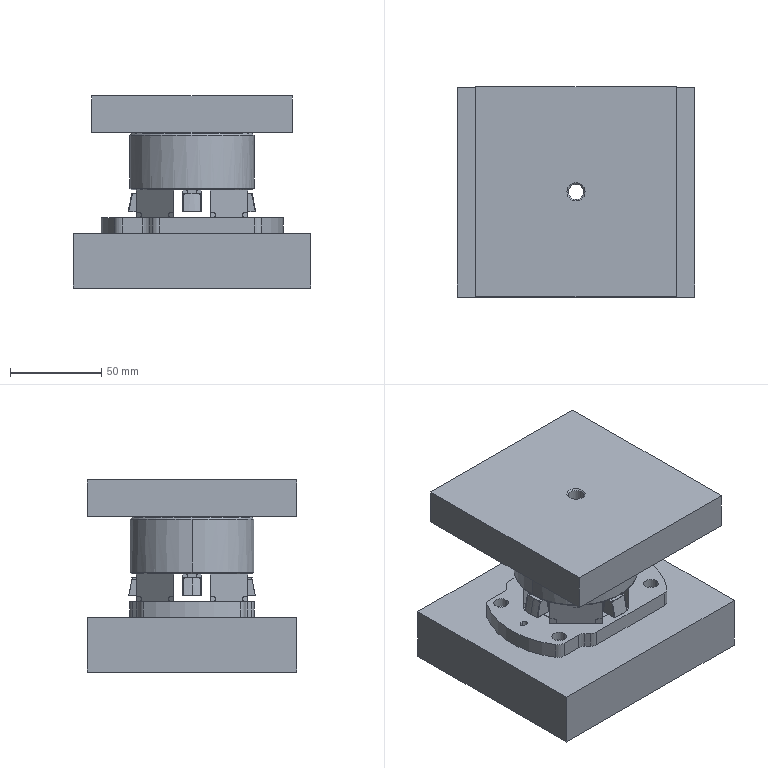NC program | NX | posted with a generic post | part box 130 x 115 x 105.2 mm
Lines 1 to 1408 of 4507:
N10 G17 G21 G94 G90
(135 , TOOL : ER25-D10-50)
N12 T04 M6
N14 G54
N16 G17 G0 G90 X-5.205 Y53.804 S5000 M3
N18 G43 Z87.387 H4
N20 G94 G1 Y7.667 Z41.249 F4500.
N22 G41 X-5.2 Y14.243 Z34.673 F2500.
N24 Y33.118 Z15.798
N26 Y34.06 Z14.855 F2292.
N28 Y35.003 Z13.913 F2083.
N30 Y35.946 Z12.97 F1875.
N32 Y36.889 Z12.027 F1667.
N34 Y37.832 Z11.084 F1458.
N36 Y38.774 Z10.141 F1250.
N38 X-10. F2500.
N40 Y37.832 Z11.084 F1250.
N42 Y36.889 Z12.027 F1667.
N44 Y35.946 Z12.97 F2083.
N46 Y14.243 Z34.673 F2500.
N48 Y7.879 Z41.037
N50 G40
N52 X-9.995 Y7.667 Z41.249
N54 X-5.205 Y6.959 Z40.542 F6000.
N56 G41 X-5.2 Y13.536 Z33.966 F2500.
N58 Y32.41 Z15.091
N60 Y33.353 Z14.148 F2292.
N62 Y34.296 Z13.206 F2083.
N64 Y35.239 Z12.263 F1875.
N66 Y36.182 Z11.32 F1667.
N68 Y37.125 Z10.377 F1458.
N70 Y38.067 Z9.434 F1250.
N72 X-10. F2500.
N74 Y37.125 Z10.377 F1250.
N76 Y36.182 Z11.32 F1667.
N78 Y35.239 Z12.263 F2083.
N80 Y13.536 Z33.966 F2500.
N82 Y7.172 Z40.33
N84 G40
N86 X-9.995 Y6.959 Z40.542
N88 X-5.205 Y6.252 Z39.835 F6000.
N90 G41 X-5.2 Y12.828 Z33.259 F2500.
N92 Y31.703 Z14.384
N94 Y32.646 Z13.441 F2292.
N96 Y33.589 Z12.498 F2083.
N98 Y34.532 Z11.556 F1875.
N100 Y35.475 Z10.613 F1667.
N102 Y36.417 Z9.67 F1458.
N104 Y37.36 Z8.727 F1250.
N106 X-10. F2500.
N108 Y36.417 Z9.67 F1250.
N110 Y35.475 Z10.613 F1667.
N112 Y34.532 Z11.556 F2083.
N114 Y12.828 Z33.259 F2500.
N116 Y6.464 Z39.623
N118 G40
N120 X-9.995 Y6.252 Z39.835
N122 X-5.205 Y5.545 Z39.128 F6000.
N124 G41 X-5.2 Y12.121 Z32.552 F2500.
N126 Y30.996 Z13.677
N128 Y31.939 Z12.734 F2292.
N130 Y32.882 Z11.791 F2083.
N132 Y33.825 Z10.849 F1875.
N134 Y34.767 Z9.906 F1667.
N136 Y35.71 Z8.963 F1458.
N138 Y36.653 Z8.02 F1250.
N140 X-10. F2500.
N142 Y35.71 Z8.963 F1250.
N144 Y34.767 Z9.906 F1667.
N146 Y33.825 Z10.849 F2083.
N148 Y12.121 Z32.552 F2500.
N150 Y5.757 Z38.916
N152 G40
N154 X-9.995 Y5.545 Z39.128
N156 X-5.205 Y4.838 Z38.421 F6000.
N158 G41 X-5.2 Y11.414 Z31.845 F2500.
N160 Y30.289 Z12.97
N162 Y31.232 Z12.027 F2292.
N164 Y32.175 Z11.084 F2083.
N166 Y33.118 Z10.141 F1875.
N168 Y34.06 Z9.199 F1667.
N170 Y35.003 Z8.256 F1458.
N172 Y35.946 Z7.313 F1250.
N174 X-10. F2500.
N176 Y35.003 Z8.256 F1250.
N178 Y34.06 Z9.199 F1667.
N180 Y33.118 Z10.141 F2083.
N182 Y11.414 Z31.845 F2500.
N184 Y5.05 Z38.209
N186 G40
N188 X-9.995 Y4.838 Z38.421
N190 X-5.205 Y4.131 Z37.714 F6000.
N192 G41 X-5.2 Y10.707 Z31.138 F2500.
N194 Y29.582 Z12.263
N196 Y30.525 Z11.32 F2292.
N198 Y31.468 Z10.377 F2083.
N200 Y32.41 Z9.434 F1875.
N202 Y33.353 Z8.492 F1667.
N204 Y34.296 Z7.549 F1458.
N206 Y35.239 Z6.606 F1250.
N208 X-10. F2500.
N210 Y34.296 Z7.549 F1250.
N212 Y33.353 Z8.492 F1667.
N214 Y32.41 Z9.434 F2083.
N216 Y10.707 Z31.138 F2500.
N218 Y4.343 Z37.502
N220 G40
N222 X-9.995 Y4.131 Z37.714
N224 X-5.205 Y3.495 Z37.077 F6000.
N226 G41 X-5.2 Y10.071 Z30.501 F2500.
N228 Y28.946 Z11.626
N230 Y29.888 Z10.684 F2292.
N232 Y30.831 Z9.741 F2083.
N234 Y31.774 Z8.798 F1875.
N236 Y32.717 Z7.855 F1667.
N238 Y33.66 Z6.912 F1458.
N240 Y34.602 Z5.969 F1250.
N242 X-10. F2500.
N244 Y33.66 Z6.912 F1250.
N246 Y32.717 Z7.855 F1667.
N248 Y31.774 Z8.798 F2083.
N250 Y10.071 Z30.501 F2500.
N252 Y3.707 Z36.865
N254 G40
N256 X-9.995 Y3.495 Z37.077
N258 G0 Y53.804 Z87.387
(PLANAR_MILL_1_5_COPY , TOOL : ER25-D10-50)
N260 X-5.205 Y-87.387
N262 Z53.804
N264 G1 Y-41.249 Z7.667 F4500.
N266 G41 X-5.2 Y-34.673 Z14.243 F2500.
N268 Y-15.798 Z33.118
N270 Y-14.855 Z34.06 F2292.
N272 Y-13.913 Z35.003 F2083.
N274 Y-12.97 Z35.946 F1875.
N276 Y-12.027 Z36.889 F1667.
N278 Y-11.084 Z37.832 F1458.
N280 Y-10.141 Z38.774 F1250.
N282 X-10. F2500.
N284 Y-11.084 Z37.832 F1250.
N286 Y-12.027 Z36.889 F1667.
N288 Y-12.97 Z35.946 F2083.
N290 Y-34.673 Z14.243 F2500.
N292 Y-41.037 Z7.879
N294 G40
N296 X-9.995 Y-41.249 Z7.667
N298 X-5.205 Y-40.542 Z6.959 F6000.
N300 G41 X-5.2 Y-33.966 Z13.536 F2500.
N302 Y-15.091 Z32.41
N304 Y-14.148 Z33.353 F2292.
N306 Y-13.206 Z34.296 F2083.
N308 Y-12.263 Z35.239 F1875.
N310 Y-11.32 Z36.182 F1667.
N312 Y-10.377 Z37.125 F1458.
N314 Y-9.434 Z38.067 F1250.
N316 X-10. F2500.
N318 Y-10.377 Z37.125 F1250.
N320 Y-11.32 Z36.182 F1667.
N322 Y-12.263 Z35.239 F2083.
N324 Y-33.966 Z13.536 F2500.
N326 Y-40.33 Z7.172
N328 G40
N330 X-9.995 Y-40.542 Z6.959
N332 X-5.205 Y-39.835 Z6.252 F6000.
N334 G41 X-5.2 Y-33.259 Z12.828 F2500.
N336 Y-14.384 Z31.703
N338 Y-13.441 Z32.646 F2292.
N340 Y-12.498 Z33.589 F2083.
N342 Y-11.556 Z34.532 F1875.
N344 Y-10.613 Z35.475 F1667.
N346 Y-9.67 Z36.417 F1458.
N348 Y-8.727 Z37.36 F1250.
N350 X-10. F2500.
N352 Y-9.67 Z36.417 F1250.
N354 Y-10.613 Z35.475 F1667.
N356 Y-11.556 Z34.532 F2083.
N358 Y-33.259 Z12.828 F2500.
N360 Y-39.623 Z6.464
N362 G40
N364 X-9.995 Y-39.835 Z6.252
N366 X-5.205 Y-39.128 Z5.545 F6000.
N368 G41 X-5.2 Y-32.552 Z12.121 F2500.
N370 Y-13.677 Z30.996
N372 Y-12.734 Z31.939 F2292.
N374 Y-11.791 Z32.882 F2083.
N376 Y-10.849 Z33.825 F1875.
N378 Y-9.906 Z34.767 F1667.
N380 Y-8.963 Z35.71 F1458.
N382 Y-8.02 Z36.653 F1250.
N384 X-10. F2500.
N386 Y-8.963 Z35.71 F1250.
N388 Y-9.906 Z34.767 F1667.
N390 Y-10.849 Z33.825 F2083.
N392 Y-32.552 Z12.121 F2500.
N394 Y-38.916 Z5.757
N396 G40
N398 X-9.995 Y-39.128 Z5.545
N400 X-5.205 Y-38.421 Z4.838 F6000.
N402 G41 X-5.2 Y-31.845 Z11.414 F2500.
N404 Y-12.97 Z30.289
N406 Y-12.027 Z31.232 F2292.
N408 Y-11.084 Z32.175 F2083.
N410 Y-10.141 Z33.118 F1875.
N412 Y-9.199 Z34.06 F1667.
N414 Y-8.256 Z35.003 F1458.
N416 Y-7.313 Z35.946 F1250.
N418 X-10. F2500.
N420 Y-8.256 Z35.003 F1250.
N422 Y-9.199 Z34.06 F1667.
N424 Y-10.141 Z33.118 F2083.
N426 Y-31.845 Z11.414 F2500.
N428 Y-38.209 Z5.05
N430 G40
N432 X-9.995 Y-38.421 Z4.838
N434 X-5.205 Y-37.714 Z4.131 F6000.
N436 G41 X-5.2 Y-31.138 Z10.707 F2500.
N438 Y-12.263 Z29.582
N440 Y-11.32 Z30.525 F2292.
N442 Y-10.377 Z31.468 F2083.
N444 Y-9.434 Z32.41 F1875.
N446 Y-8.492 Z33.353 F1667.
N448 Y-7.549 Z34.296 F1458.
N450 Y-6.606 Z35.239 F1250.
N452 X-10. F2500.
N454 Y-7.549 Z34.296 F1250.
N456 Y-8.492 Z33.353 F1667.
N458 Y-9.434 Z32.41 F2083.
N460 Y-31.138 Z10.707 F2500.
N462 Y-37.502 Z4.343
N464 G40
N466 X-9.995 Y-37.714 Z4.131
N468 X-5.205 Y-37.077 Z3.495 F6000.
N470 G41 X-5.2 Y-30.501 Z10.071 F2500.
N472 Y-11.626 Z28.946
N474 Y-10.684 Z29.888 F2292.
N476 Y-9.741 Z30.831 F2083.
N478 Y-8.798 Z31.774 F1875.
N480 Y-7.855 Z32.717 F1667.
N482 Y-6.912 Z33.66 F1458.
N484 Y-5.969 Z34.602 F1250.
N486 X-10. F2500.
N488 Y-6.912 Z33.66 F1250.
N490 Y-7.855 Z32.717 F1667.
N492 Y-8.798 Z31.774 F2083.
N494 Y-30.501 Z10.071 F2500.
N496 Y-36.865 Z3.707
N498 G40
N500 X-9.995 Y-37.077 Z3.495
N502 G0 Y-87.387 Z53.804
(PLANAR_MILL_1_5_COPY_1 , TOOL : ER25-D10-50)
N504 X-5.205 Y-53.804
N506 Z-87.387
N508 G1 Y-7.667 Z-41.249 F4500.
N510 G41 X-5.2 Y-14.243 Z-34.673 F2500.
N512 Y-33.118 Z-15.798
N514 Y-34.06 Z-14.855 F2292.
N516 Y-35.003 Z-13.913 F2083.
N518 Y-35.946 Z-12.97 F1875.
N520 Y-36.889 Z-12.027 F1667.
N522 Y-37.832 Z-11.084 F1458.
N524 Y-38.774 Z-10.141 F1250.
N526 X-10. F2500.
N528 Y-37.832 Z-11.084 F1250.
N530 Y-36.889 Z-12.027 F1667.
N532 Y-35.946 Z-12.97 F2083.
N534 Y-14.243 Z-34.673 F2500.
N536 Y-7.879 Z-41.037
N538 G40
N540 X-9.995 Y-7.667 Z-41.249
N542 X-5.205 Y-6.959 Z-40.542 F6000.
N544 G41 X-5.2 Y-13.536 Z-33.966 F2500.
N546 Y-32.41 Z-15.091
N548 Y-33.353 Z-14.148 F2292.
N550 Y-34.296 Z-13.206 F2083.
N552 Y-35.239 Z-12.263 F1875.
N554 Y-36.182 Z-11.32 F1667.
N556 Y-37.125 Z-10.377 F1458.
N558 Y-38.067 Z-9.434 F1250.
N560 X-10. F2500.
N562 Y-37.125 Z-10.377 F1250.
N564 Y-36.182 Z-11.32 F1667.
N566 Y-35.239 Z-12.263 F2083.
N568 Y-13.536 Z-33.966 F2500.
N570 Y-7.172 Z-40.33
N572 G40
N574 X-9.995 Y-6.959 Z-40.542
N576 X-5.205 Y-6.252 Z-39.835 F6000.
N578 G41 X-5.2 Y-12.828 Z-33.259 F2500.
N580 Y-31.703 Z-14.384
N582 Y-32.646 Z-13.441 F2292.
N584 Y-33.589 Z-12.498 F2083.
N586 Y-34.532 Z-11.556 F1875.
N588 Y-35.475 Z-10.613 F1667.
N590 Y-36.417 Z-9.67 F1458.
N592 Y-37.36 Z-8.727 F1250.
N594 X-10. F2500.
N596 Y-36.417 Z-9.67 F1250.
N598 Y-35.475 Z-10.613 F1667.
N600 Y-34.532 Z-11.556 F2083.
N602 Y-12.828 Z-33.259 F2500.
N604 Y-6.464 Z-39.623
N606 G40
N608 X-9.995 Y-6.252 Z-39.835
N610 X-5.205 Y-5.545 Z-39.128 F6000.
N612 G41 X-5.2 Y-12.121 Z-32.552 F2500.
N614 Y-30.996 Z-13.677
N616 Y-31.939 Z-12.734 F2292.
N618 Y-32.882 Z-11.791 F2083.
N620 Y-33.825 Z-10.849 F1875.
N622 Y-34.767 Z-9.906 F1667.
N624 Y-35.71 Z-8.963 F1458.
N626 Y-36.653 Z-8.02 F1250.
N628 X-10. F2500.
N630 Y-35.71 Z-8.963 F1250.
N632 Y-34.767 Z-9.906 F1667.
N634 Y-33.825 Z-10.849 F2083.
N636 Y-12.121 Z-32.552 F2500.
N638 Y-5.757 Z-38.916
N640 G40
N642 X-9.995 Y-5.545 Z-39.128
N644 X-5.205 Y-4.838 Z-38.421 F6000.
N646 G41 X-5.2 Y-11.414 Z-31.845 F2500.
N648 Y-30.289 Z-12.97
N650 Y-31.232 Z-12.027 F2292.
N652 Y-32.175 Z-11.084 F2083.
N654 Y-33.118 Z-10.141 F1875.
N656 Y-34.06 Z-9.199 F1667.
N658 Y-35.003 Z-8.256 F1458.
N660 Y-35.946 Z-7.313 F1250.
N662 X-10. F2500.
N664 Y-35.003 Z-8.256 F1250.
N666 Y-34.06 Z-9.199 F1667.
N668 Y-33.118 Z-10.141 F2083.
N670 Y-11.414 Z-31.845 F2500.
N672 Y-5.05 Z-38.209
N674 G40
N676 X-9.995 Y-4.838 Z-38.421
N678 X-5.205 Y-4.131 Z-37.714 F6000.
N680 G41 X-5.2 Y-10.707 Z-31.138 F2500.
N682 Y-29.582 Z-12.263
N684 Y-30.525 Z-11.32 F2292.
N686 Y-31.468 Z-10.377 F2083.
N688 Y-32.41 Z-9.434 F1875.
N690 Y-33.353 Z-8.492 F1667.
N692 Y-34.296 Z-7.549 F1458.
N694 Y-35.239 Z-6.606 F1250.
N696 X-10. F2500.
N698 Y-34.296 Z-7.549 F1250.
N700 Y-33.353 Z-8.492 F1667.
N702 Y-32.41 Z-9.434 F2083.
N704 Y-10.707 Z-31.138 F2500.
N706 Y-4.343 Z-37.502
N708 G40
N710 X-9.995 Y-4.131 Z-37.714
N712 X-5.205 Y-3.495 Z-37.077 F6000.
N714 G41 X-5.2 Y-10.071 Z-30.501 F2500.
N716 Y-28.946 Z-11.626
N718 Y-29.888 Z-10.684 F2292.
N720 Y-30.831 Z-9.741 F2083.
N722 Y-31.774 Z-8.798 F1875.
N724 Y-32.717 Z-7.855 F1667.
N726 Y-33.66 Z-6.912 F1458.
N728 Y-34.602 Z-5.969 F1250.
N730 X-10. F2500.
N732 Y-33.66 Z-6.912 F1250.
N734 Y-32.717 Z-7.855 F1667.
N736 Y-31.774 Z-8.798 F2083.
N738 Y-10.071 Z-30.501 F2500.
N740 Y-3.707 Z-36.865
N742 G40
N744 X-9.995 Y-3.495 Z-37.077
N746 G0 Y-53.804 Z-87.387
(PLANAR_MILL_1_5_COPY_2 , TOOL : ER25-D10-50)
N748 Z-53.804
N750 X-5.205 Y87.387
N752 G1 Y41.249 Z-7.667 F4500.
N754 G41 X-5.2 Y34.673 Z-14.243 F2500.
N756 Y15.798 Z-33.118
N758 Y14.855 Z-34.06 F2292.
N760 Y13.913 Z-35.003 F2083.
N762 Y12.97 Z-35.946 F1875.
N764 Y12.027 Z-36.889 F1667.
N766 Y11.084 Z-37.832 F1458.
N768 Y10.141 Z-38.774 F1250.
N770 X-10. F2500.
N772 Y11.084 Z-37.832 F1250.
N774 Y12.027 Z-36.889 F1667.
N776 Y12.97 Z-35.946 F2083.
N778 Y34.673 Z-14.243 F2500.
N780 Y41.037 Z-7.879
N782 G40
N784 X-9.995 Y41.249 Z-7.667
N786 X-5.205 Y40.542 Z-6.959 F6000.
N788 G41 X-5.2 Y33.966 Z-13.536 F2500.
N790 Y15.091 Z-32.41
N792 Y14.148 Z-33.353 F2292.
N794 Y13.206 Z-34.296 F2083.
N796 Y12.263 Z-35.239 F1875.
N798 Y11.32 Z-36.182 F1667.
N800 Y10.377 Z-37.125 F1458.
N802 Y9.434 Z-38.067 F1250.
N804 X-10. F2500.
N806 Y10.377 Z-37.125 F1250.
N808 Y11.32 Z-36.182 F1667.
N810 Y12.263 Z-35.239 F2083.
N812 Y33.966 Z-13.536 F2500.
N814 Y40.33 Z-7.172
N816 G40
N818 X-9.995 Y40.542 Z-6.959
N820 X-5.205 Y39.835 Z-6.252 F6000.
N822 G41 X-5.2 Y33.259 Z-12.828 F2500.
N824 Y14.384 Z-31.703
N826 Y13.441 Z-32.646 F2292.
N828 Y12.498 Z-33.589 F2083.
N830 Y11.556 Z-34.532 F1875.
N832 Y10.613 Z-35.475 F1667.
N834 Y9.67 Z-36.417 F1458.
N836 Y8.727 Z-37.36 F1250.
N838 X-10. F2500.
N840 Y9.67 Z-36.417 F1250.
N842 Y10.613 Z-35.475 F1667.
N844 Y11.556 Z-34.532 F2083.
N846 Y33.259 Z-12.828 F2500.
N848 Y39.623 Z-6.464
N850 G40
N852 X-9.995 Y39.835 Z-6.252
N854 X-5.205 Y39.128 Z-5.545 F6000.
N856 G41 X-5.2 Y32.552 Z-12.121 F2500.
N858 Y13.677 Z-30.996
N860 Y12.734 Z-31.939 F2292.
N862 Y11.791 Z-32.882 F2083.
N864 Y10.849 Z-33.825 F1875.
N866 Y9.906 Z-34.767 F1667.
N868 Y8.963 Z-35.71 F1458.
N870 Y8.02 Z-36.653 F1250.
N872 X-10. F2500.
N874 Y8.963 Z-35.71 F1250.
N876 Y9.906 Z-34.767 F1667.
N878 Y10.849 Z-33.825 F2083.
N880 Y32.552 Z-12.121 F2500.
N882 Y38.916 Z-5.757
N884 G40
N886 X-9.995 Y39.128 Z-5.545
N888 X-5.205 Y38.421 Z-4.838 F6000.
N890 G41 X-5.2 Y31.845 Z-11.414 F2500.
N892 Y12.97 Z-30.289
N894 Y12.027 Z-31.232 F2292.
N896 Y11.084 Z-32.175 F2083.
N898 Y10.141 Z-33.118 F1875.
N900 Y9.199 Z-34.06 F1667.
N902 Y8.256 Z-35.003 F1458.
N904 Y7.313 Z-35.946 F1250.
N906 X-10. F2500.
N908 Y8.256 Z-35.003 F1250.
N910 Y9.199 Z-34.06 F1667.
N912 Y10.141 Z-33.118 F2083.
N914 Y31.845 Z-11.414 F2500.
N916 Y38.209 Z-5.05
N918 G40
N920 X-9.995 Y38.421 Z-4.838
N922 X-5.205 Y37.714 Z-4.131 F6000.
N924 G41 X-5.2 Y31.138 Z-10.707 F2500.
N926 Y12.263 Z-29.582
N928 Y11.32 Z-30.525 F2292.
N930 Y10.377 Z-31.468 F2083.
N932 Y9.434 Z-32.41 F1875.
N934 Y8.492 Z-33.353 F1667.
N936 Y7.549 Z-34.296 F1458.
N938 Y6.606 Z-35.239 F1250.
N940 X-10. F2500.
N942 Y7.549 Z-34.296 F1250.
N944 Y8.492 Z-33.353 F1667.
N946 Y9.434 Z-32.41 F2083.
N948 Y31.138 Z-10.707 F2500.
N950 Y37.502 Z-4.343
N952 G40
N954 X-9.995 Y37.714 Z-4.131
N956 X-5.205 Y37.077 Z-3.495 F6000.
N958 G41 X-5.2 Y30.501 Z-10.071 F2500.
N960 Y11.626 Z-28.946
N962 Y10.684 Z-29.888 F2292.
N964 Y9.741 Z-30.831 F2083.
N966 Y8.798 Z-31.774 F1875.
N968 Y7.855 Z-32.717 F1667.
N970 Y6.912 Z-33.66 F1458.
N972 Y5.969 Z-34.602 F1250.
N974 X-10. F2500.
N976 Y6.912 Z-33.66 F1250.
N978 Y7.855 Z-32.717 F1667.
N980 Y8.798 Z-31.774 F2083.
N982 Y30.501 Z-10.071 F2500.
N984 Y36.865 Z-3.707
N986 G40
N988 X-9.995 Y37.077 Z-3.495
N990 G0 Y87.387 Z-53.804
N992 M5
(136 , TOOL : ER25-D10-50_G)
N994 T05 M6
N996 G54
N998 G17 G0 G90 X-5.053 Y53.875 S5000 M3
N1000 G43 Z87.316 H5
N1002 G94 G1 Y3.495 Z36.936 F4500.
N1004 G41 X-5.05 Y10. Z30.431 F1000. D5
N1006 Y28.981 Z11.45
N1008 Y29.924 Z10.507 F917.
N1010 Y30.867 Z9.564 F833.
N1012 Y31.809 Z8.621 F750.
N1014 Y32.752 Z7.678 F667.
N1016 Y33.695 Z6.736 F583.
N1018 Y34.638 Z5.793 F500.
N1020 X-10.15 F1000.
N1022 Y33.695 Z6.736 F500.
N1024 Y32.752 Z7.678 F667.
N1026 Y31.809 Z8.621 F833.
N1028 Y10. Z30.431 F1000.
N1030 Y3.636 Z36.795
N1032 G40
N1034 X-10.147 Y3.495 Z36.936
N1036 G0 Y53.875 Z87.316
(PLANAR_MILL_1_5_COPY_3_COPY , TOOL : ER25-D10-50_G)
N1038 X-5.055 Y-87.387
N1040 Z53.804
N1042 G1 Y-37.007 Z3.424 F4500.
N1044 G41 X-5.05 Y-30.431 Z10. F1000.
N1046 Y-11.45 Z28.981
N1048 Y-10.507 Z29.924 F917.
N1050 Y-9.564 Z30.867 F833.
N1052 Y-8.621 Z31.809 F750.
N1054 Y-7.678 Z32.752 F667.
N1056 Y-6.736 Z33.695 F583.
N1058 Y-5.793 Z34.638 F500.
N1060 X-10.15 F1000.
N1062 Y-6.736 Z33.695 F500.
N1064 Y-7.678 Z32.752 F667.
N1066 Y-8.621 Z31.809 F833.
N1068 Y-30.431 Z10. F1000.
N1070 Y-36.795 Z3.636
N1072 G40
N1074 X-10.145 Y-37.007 Z3.424
N1076 G0 Y-87.387 Z53.804
(PLANAR_MILL_1_5_COPY_3_COPY_1 , TOOL : ER25-D10-50_G)
N1078 X-5.055 Y-53.804
N1080 Z-87.387
N1082 G1 Y-3.424 Z-37.007 F4500.
N1084 G41 X-5.05 Y-10. Z-30.431 F1000.
N1086 Y-28.981 Z-11.45
N1088 Y-29.924 Z-10.507 F917.
N1090 Y-30.867 Z-9.564 F833.
N1092 Y-31.809 Z-8.621 F750.
N1094 Y-32.752 Z-7.678 F667.
N1096 Y-33.695 Z-6.736 F583.
N1098 Y-34.638 Z-5.793 F500.
N1100 X-10.15 F1000.
N1102 Y-33.695 Z-6.736 F500.
N1104 Y-32.752 Z-7.678 F667.
N1106 Y-31.809 Z-8.621 F833.
N1108 Y-10. Z-30.431 F1000.
N1110 Y-3.636 Z-36.795
N1112 G40
N1114 X-10.145 Y-3.424 Z-37.007
N1116 G0 Y-53.804 Z-87.387
(PLANAR_MILL_1_5_COPY_3_COPY_2 , TOOL : ER25-D10-50_G)
N1118 Z-53.804
N1120 X-5.055 Y87.387
N1122 G1 Y37.007 Z-3.424 F4500.
N1124 G41 X-5.05 Y30.431 Z-10. F1000.
N1126 Y11.45 Z-28.981
N1128 Y10.507 Z-29.924 F917.
N1130 Y9.564 Z-30.867 F833.
N1132 Y8.621 Z-31.809 F750.
N1134 Y7.678 Z-32.752 F667.
N1136 Y6.736 Z-33.695 F583.
N1138 Y5.793 Z-34.638 F500.
N1140 X-10.15 F1000.
N1142 Y6.736 Z-33.695 F500.
N1144 Y7.678 Z-32.752 F667.
N1146 Y8.621 Z-31.809 F833.
N1148 Y30.431 Z-10. F1000.
N1150 Y36.795 Z-3.636
N1152 G40
N1154 X-10.145 Y37.007 Z-3.424
N1156 G0 Y87.387 Z-53.804
N1158 M5
(137 , TOOL : ER25-D1.5-23)
N1160 T16 M6
N1162 G54
N1164 G17 G0 G90 X-14.35 Y-5.492 S5000 M3
N1166 G43 Z85. H16
N1168 G94 G1 Z35. F4500.
N1170 Y-6.15 Z34.994 F1200.
N1172 X-14.05 Z34.992
N1174 Y6.15 Z34.884
N1176 X-14.35 Z34.882
N1178 Y-6.15 Z34.774
N1180 X-14.05 Z34.772
N1182 Y6.15 Z34.664
N1184 X-14.35 Z34.662
N1186 Y-6.15 Z34.554
N1188 X-14.05 Z34.552
N1190 Y6.15 Z34.444
N1192 X-14.35 Z34.442
N1194 Y-6.15 Z34.335
N1196 X-14.05 Z34.332
N1198 Y6.15 Z34.225
N1200 X-14.35 Z34.222
N1202 Y-6.15 Z34.115
N1204 X-14.05 Z34.112
N1206 Y6.15 Z34.005
N1208 X-14.35 Z34.002
N1210 Y-6.15 Z33.895
N1212 X-14.05 Z33.892
N1214 Y6.15 Z33.785
N1216 X-14.35 Z33.782
N1218 Y-6.15 Z33.675
N1220 X-14.05 Z33.672
N1222 Y6.15 Z33.565
N1224 X-14.35 Z33.562
N1226 Y-6.15 Z33.455
N1228 X-14.05 Z33.452
N1230 Y6.15 Z33.345
N1232 X-14.35 Z33.342
N1234 Y-6.15 Z33.235
N1236 X-14.05 Z33.232
N1238 Y6.15 Z33.125
N1240 X-14.35 Z33.122
N1242 Y-6.15 Z33.015
N1244 X-14.05 Z33.012
N1246 Y6.15 Z32.905
N1248 X-14.35 Z32.902
N1250 Y-6.15 Z32.795
N1252 X-14.05 Z32.792
N1254 Y6.15 Z32.685
N1256 X-14.35 Z32.683
N1258 Y-6.15 Z32.575
N1260 X-14.05 Z32.573
N1262 Y6.15 Z32.465
N1264 X-14.35 Z32.463
N1266 Y-6.15 Z32.355
N1268 X-14.05 Z32.353
N1270 Y6.15 Z32.245
N1272 X-14.35 Z32.243
N1274 Y-6.15 Z32.135
N1276 X-14.05 Z32.133
N1278 Y6.15 Z32.025
N1280 X-14.35 Z32.023
N1282 Y-6.15 Z31.915
N1284 X-14.05 Z31.913
N1286 Y6.15 Z31.805
N1288 X-14.35 Z31.803
N1290 Y-6.15 Z31.696
N1292 X-14.05 Z31.693
N1294 Y6.15 Z31.586
N1296 X-14.35 Z31.583
N1298 Y-6.15 Z31.476
N1300 X-14.05 Z31.473
N1302 Y6.15 Z31.366
N1304 X-14.35 Z31.363
N1306 Y-6.15 Z31.256
N1308 X-14.05 Z31.253
N1310 Y6.15 Z31.146
N1312 X-14.35 Z31.143
N1314 Y-6.15 Z31.036
N1316 X-14.05 Z31.033
N1318 Y6.15 Z30.926
N1320 X-14.35 Z30.923
N1322 Y-6.15 Z30.816
N1324 X-14.05 Z30.813
N1326 Y6.15 Z30.706
N1328 X-14.35 Z30.703
N1330 Y-6.15 Z30.596
N1332 X-14.05 Z30.593
N1334 Y6.15 Z30.486
N1336 X-14.35 Z30.483
N1338 Y-6.15 Z30.376
N1340 X-14.05 Z30.373
N1342 Y6.15 Z30.266
N1344 X-14.35 Z30.263
N1346 Y-6.15 Z30.156
N1348 X-14.05 Z30.153
N1350 Y6.15 Z30.046
N1352 X-14.35 Z30.044
N1354 Y-6.15 Z29.936
N1356 X-14.05 Z29.934
N1358 Y6.15 Z29.826
N1360 X-14.35 Z29.824
N1362 Y-6.15 Z29.716
N1364 X-14.05 Z29.714
N1366 Y6.15 Z29.606
N1368 X-14.35 Z29.604
N1370 Y0. Z29.55
N1372 Y-4.95
N1374 Y-5.15 F1100.
N1376 Y-5.35 F1000.
N1378 Y-5.55 F900.
N1380 Y-5.75 F800.
N1382 Y-5.95 F700.
N1384 Y-6.15 F600.
N1386 X-14.05 F1200.
N1388 Y-5.95 F600.
N1390 Y-5.75 F800.
N1392 Y-5.55 F1000.
N1394 Y4.95 F1200.
N1396 Y5.15 F1100.
N1398 Y5.35 F1000.
N1400 Y5.55 F900.
N1402 Y5.75 F800.
N1404 Y5.95 F700.
N1406 Y6.15 F600.
N1408 X-14.35 F1200.
N1410 Y5.95 F600.
N1412 Y5.75 F800.
N1414 Y5.55 F1000.
N1416 Y0. F1200.
N1418 Y-0.5
N1420 Z30.05
N1422 G0 Z85.
(PLANAR_MILL_1_5_COPY_4_COPY_1 , TOOL : ER25-D1.5-23)
N1424 G18 X-14.35 Z-5.492
N1426 Y-85.
N1428 G1 Y-35. F4500.
N1430 Y-34.994 Z-6.15 F1200.
N1432 X-14.05 Y-34.992
N1434 Y-34.884 Z6.15
N1436 X-14.35 Y-34.882
N1438 Y-34.774 Z-6.15
N1440 X-14.05 Y-34.772
N1442 Y-34.664 Z6.15
N1444 X-14.35 Y-34.662
N1446 Y-34.554 Z-6.15
N1448 X-14.05 Y-34.552
N1450 Y-34.444 Z6.15
N1452 X-14.35 Y-34.442
N1454 Y-34.335 Z-6.15
N1456 X-14.05 Y-34.332
N1458 Y-34.225 Z6.15
N1460 X-14.35 Y-34.222
N1462 Y-34.115 Z-6.15
N1464 X-14.05 Y-34.112
N1466 Y-34.005 Z6.15
N1468 X-14.35 Y-34.002
N1470 Y-33.895 Z-6.15
N1472 X-14.05 Y-33.892
N1474 Y-33.785 Z6.15
N1476 X-14.35 Y-33.782
N1478 Y-33.675 Z-6.15
N1480 X-14.05 Y-33.672
N1482 Y-33.565 Z6.15
N1484 X-14.35 Y-33.562
N1486 Y-33.455 Z-6.15
N1488 X-14.05 Y-33.452
N1490 Y-33.345 Z6.15
N1492 X-14.35 Y-33.342
N1494 Y-33.235 Z-6.15
N1496 X-14.05 Y-33.232
N1498 Y-33.125 Z6.15
N1500 X-14.35 Y-33.122
N1502 Y-33.015 Z-6.15
N1504 X-14.05 Y-33.012
N1506 Y-32.905 Z6.15
N1508 X-14.35 Y-32.902
N1510 Y-32.795 Z-6.15
N1512 X-14.05 Y-32.792
N1514 Y-32.685 Z6.15
N1516 X-14.35 Y-32.683
N1518 Y-32.575 Z-6.15
N1520 X-14.05 Y-32.573
N1522 Y-32.465 Z6.15
N1524 X-14.35 Y-32.463
N1526 Y-32.355 Z-6.15
N1528 X-14.05 Y-32.353
N1530 Y-32.245 Z6.15
N1532 X-14.35 Y-32.243
N1534 Y-32.135 Z-6.15
N1536 X-14.05 Y-32.133
N1538 Y-32.025 Z6.15
N1540 X-14.35 Y-32.023
N1542 Y-31.915 Z-6.15
N1544 X-14.05 Y-31.913
N1546 Y-31.805 Z6.15
N1548 X-14.35 Y-31.803
N1550 Y-31.696 Z-6.15
N1552 X-14.05 Y-31.693
N1554 Y-31.586 Z6.15
N1556 X-14.35 Y-31.583
N1558 Y-31.476 Z-6.15
N1560 X-14.05 Y-31.473
N1562 Y-31.366 Z6.15
N1564 X-14.35 Y-31.363
N1566 Y-31.256 Z-6.15
N1568 X-14.05 Y-31.253
N1570 Y-31.146 Z6.15
N1572 X-14.35 Y-31.143
N1574 Y-31.036 Z-6.15
N1576 X-14.05 Y-31.033
N1578 Y-30.926 Z6.15
N1580 X-14.35 Y-30.923
N1582 Y-30.816 Z-6.15
N1584 X-14.05 Y-30.813
N1586 Y-30.706 Z6.15
N1588 X-14.35 Y-30.703
N1590 Y-30.596 Z-6.15
N1592 X-14.05 Y-30.593
N1594 Y-30.486 Z6.15
N1596 X-14.35 Y-30.483
N1598 Y-30.376 Z-6.15
N1600 X-14.05 Y-30.373
N1602 Y-30.266 Z6.15
N1604 X-14.35 Y-30.263
N1606 Y-30.156 Z-6.15
N1608 X-14.05 Y-30.153
N1610 Y-30.046 Z6.15
N1612 X-14.35 Y-30.044
N1614 Y-29.936 Z-6.15
N1616 X-14.05 Y-29.934
N1618 Y-29.826 Z6.15
N1620 X-14.35 Y-29.824
N1622 Y-29.716 Z-6.15
N1624 X-14.05 Y-29.714
N1626 Y-29.606 Z6.15
N1628 X-14.35 Y-29.604
N1630 Y-29.55 Z0.
N1632 Z-4.95
N1634 Z-5.15 F1100.
N1636 Z-5.35 F1000.
N1638 Z-5.55 F900.
N1640 Z-5.75 F800.
N1642 Z-5.95 F700.
N1644 Z-6.15 F600.
N1646 X-14.05 F1200.
N1648 Z-5.95 F600.
N1650 Z-5.75 F800.
N1652 Z-5.55 F1000.
N1654 Z4.95 F1200.
N1656 Z5.15 F1100.
N1658 Z5.35 F1000.
N1660 Z5.55 F900.
N1662 Z5.75 F800.
N1664 Z5.95 F700.
N1666 Z6.15 F600.
N1668 X-14.35 F1200.
N1670 Z5.95 F600.
N1672 Z5.75 F800.
N1674 Z5.55 F1000.
N1676 Z0. F1200.
N1678 Z-0.5
N1680 Y-30.05
N1682 G0 Y-85.
(PLANAR_MILL_1_5_COPY_4_COPY_2 , TOOL : ER25-D1.5-23)
N1684 G17 X-14.35 Y5.492
N1686 Z-85.
N1688 G1 Z-35. F4500.
N1690 Y6.15 Z-34.994 F1200.
N1692 X-14.05 Z-34.992
N1694 Y-6.15 Z-34.884
N1696 X-14.35 Z-34.882
N1698 Y6.15 Z-34.774
N1700 X-14.05 Z-34.772
N1702 Y-6.15 Z-34.664
N1704 X-14.35 Z-34.662
N1706 Y6.15 Z-34.554
N1708 X-14.05 Z-34.552
N1710 Y-6.15 Z-34.444
N1712 X-14.35 Z-34.442
N1714 Y6.15 Z-34.335
N1716 X-14.05 Z-34.332
N1718 Y-6.15 Z-34.225
N1720 X-14.35 Z-34.222
N1722 Y6.15 Z-34.115
N1724 X-14.05 Z-34.112
N1726 Y-6.15 Z-34.005
N1728 X-14.35 Z-34.002
N1730 Y6.15 Z-33.895
N1732 X-14.05 Z-33.892
N1734 Y-6.15 Z-33.785
N1736 X-14.35 Z-33.782
N1738 Y6.15 Z-33.675
N1740 X-14.05 Z-33.672
N1742 Y-6.15 Z-33.565
N1744 X-14.35 Z-33.562
N1746 Y6.15 Z-33.455
N1748 X-14.05 Z-33.452
N1750 Y-6.15 Z-33.345
N1752 X-14.35 Z-33.342
N1754 Y6.15 Z-33.235
N1756 X-14.05 Z-33.232
N1758 Y-6.15 Z-33.125
N1760 X-14.35 Z-33.122
N1762 Y6.15 Z-33.015
N1764 X-14.05 Z-33.012
N1766 Y-6.15 Z-32.905
N1768 X-14.35 Z-32.902
N1770 Y6.15 Z-32.795
N1772 X-14.05 Z-32.792
N1774 Y-6.15 Z-32.685
N1776 X-14.35 Z-32.683
N1778 Y6.15 Z-32.575
N1780 X-14.05 Z-32.573
N1782 Y-6.15 Z-32.465
N1784 X-14.35 Z-32.463
N1786 Y6.15 Z-32.355
N1788 X-14.05 Z-32.353
N1790 Y-6.15 Z-32.245
N1792 X-14.35 Z-32.243
N1794 Y6.15 Z-32.135
N1796 X-14.05 Z-32.133
N1798 Y-6.15 Z-32.025
N1800 X-14.35 Z-32.023
N1802 Y6.15 Z-31.915
N1804 X-14.05 Z-31.913
N1806 Y-6.15 Z-31.805
N1808 X-14.35 Z-31.803
N1810 Y6.15 Z-31.696
N1812 X-14.05 Z-31.693
N1814 Y-6.15 Z-31.586
N1816 X-14.35 Z-31.583
N1818 Y6.15 Z-31.476
N1820 X-14.05 Z-31.473
N1822 Y-6.15 Z-31.366
N1824 X-14.35 Z-31.363
N1826 Y6.15 Z-31.256
N1828 X-14.05 Z-31.253
N1830 Y-6.15 Z-31.146
N1832 X-14.35 Z-31.143
N1834 Y6.15 Z-31.036
N1836 X-14.05 Z-31.033
N1838 Y-6.15 Z-30.926
N1840 X-14.35 Z-30.923
N1842 Y6.15 Z-30.816
N1844 X-14.05 Z-30.813
N1846 Y-6.15 Z-30.706
N1848 X-14.35 Z-30.703
N1850 Y6.15 Z-30.596
N1852 X-14.05 Z-30.593
N1854 Y-6.15 Z-30.486
N1856 X-14.35 Z-30.483
N1858 Y6.15 Z-30.376
N1860 X-14.05 Z-30.373
N1862 Y-6.15 Z-30.266
N1864 X-14.35 Z-30.263
N1866 Y6.15 Z-30.156
N1868 X-14.05 Z-30.153
N1870 Y-6.15 Z-30.046
N1872 X-14.35 Z-30.044
N1874 Y6.15 Z-29.936
N1876 X-14.05 Z-29.934
N1878 Y-6.15 Z-29.826
N1880 X-14.35 Z-29.824
N1882 Y6.15 Z-29.716
N1884 X-14.05 Z-29.714
N1886 Y-6.15 Z-29.606
N1888 X-14.35 Z-29.604
N1890 Y0. Z-29.55
N1892 Y4.95
N1894 Y5.15 F1100.
N1896 Y5.35 F1000.
N1898 Y5.55 F900.
N1900 Y5.75 F800.
N1902 Y5.95 F700.
N1904 Y6.15 F600.
N1906 X-14.05 F1200.
N1908 Y5.95 F600.
N1910 Y5.75 F800.
N1912 Y5.55 F1000.
N1914 Y-4.95 F1200.
N1916 Y-5.15 F1100.
N1918 Y-5.35 F1000.
N1920 Y-5.55 F900.
N1922 Y-5.75 F800.
N1924 Y-5.95 F700.
N1926 Y-6.15 F600.
N1928 X-14.35 F1200.
N1930 Y-5.95 F600.
N1932 Y-5.75 F800.
N1934 Y-5.55 F1000.
N1936 Y0. F1200.
N1938 Y0.5
N1940 Z-30.05
N1942 G0 Z-85.
(PLANAR_MILL_1_5_COPY_4_COPY_3 , TOOL : ER25-D1.5-23)
N1944 G18 Y85.
N1946 X-14.35 Z5.492
N1948 G1 Y35. F4500.
N1950 Y34.994 Z6.15 F1200.
N1952 X-14.05 Y34.992
N1954 Y34.884 Z-6.15
N1956 X-14.35 Y34.882
N1958 Y34.774 Z6.15
N1960 X-14.05 Y34.772
N1962 Y34.664 Z-6.15
N1964 X-14.35 Y34.662
N1966 Y34.554 Z6.15
N1968 X-14.05 Y34.552
N1970 Y34.444 Z-6.15
N1972 X-14.35 Y34.442
N1974 Y34.335 Z6.15
N1976 X-14.05 Y34.332
N1978 Y34.225 Z-6.15
N1980 X-14.35 Y34.222
N1982 Y34.115 Z6.15
N1984 X-14.05 Y34.112
N1986 Y34.005 Z-6.15
N1988 X-14.35 Y34.002
N1990 Y33.895 Z6.15
N1992 X-14.05 Y33.892
N1994 Y33.785 Z-6.15
N1996 X-14.35 Y33.782
N1998 Y33.675 Z6.15
N2000 X-14.05 Y33.672
N2002 Y33.565 Z-6.15
N2004 X-14.35 Y33.562
N2006 Y33.455 Z6.15
N2008 X-14.05 Y33.452
N2010 Y33.345 Z-6.15
N2012 X-14.35 Y33.342
N2014 Y33.235 Z6.15
N2016 X-14.05 Y33.232
N2018 Y33.125 Z-6.15
N2020 X-14.35 Y33.122
N2022 Y33.015 Z6.15
N2024 X-14.05 Y33.012
N2026 Y32.905 Z-6.15
N2028 X-14.35 Y32.902
N2030 Y32.795 Z6.15
N2032 X-14.05 Y32.792
N2034 Y32.685 Z-6.15
N2036 X-14.35 Y32.683
N2038 Y32.575 Z6.15
N2040 X-14.05 Y32.573
N2042 Y32.465 Z-6.15
N2044 X-14.35 Y32.463
N2046 Y32.355 Z6.15
N2048 X-14.05 Y32.353
N2050 Y32.245 Z-6.15
N2052 X-14.35 Y32.243
N2054 Y32.135 Z6.15
N2056 X-14.05 Y32.133
N2058 Y32.025 Z-6.15
N2060 X-14.35 Y32.023
N2062 Y31.915 Z6.15
N2064 X-14.05 Y31.913
N2066 Y31.805 Z-6.15
N2068 X-14.35 Y31.803
N2070 Y31.696 Z6.15
N2072 X-14.05 Y31.693
N2074 Y31.586 Z-6.15
N2076 X-14.35 Y31.583
N2078 Y31.476 Z6.15
N2080 X-14.05 Y31.473
N2082 Y31.366 Z-6.15
N2084 X-14.35 Y31.363
N2086 Y31.256 Z6.15
N2088 X-14.05 Y31.253
N2090 Y31.146 Z-6.15
N2092 X-14.35 Y31.143
N2094 Y31.036 Z6.15
N2096 X-14.05 Y31.033
N2098 Y30.926 Z-6.15
N2100 X-14.35 Y30.923
N2102 Y30.816 Z6.15
N2104 X-14.05 Y30.813
N2106 Y30.706 Z-6.15
N2108 X-14.35 Y30.703
N2110 Y30.596 Z6.15
N2112 X-14.05 Y30.593
N2114 Y30.486 Z-6.15
N2116 X-14.35 Y30.483
N2118 Y30.376 Z6.15
N2120 X-14.05 Y30.373
N2122 Y30.266 Z-6.15
N2124 X-14.35 Y30.263
N2126 Y30.156 Z6.15
N2128 X-14.05 Y30.153
N2130 Y30.046 Z-6.15
N2132 X-14.35 Y30.044
N2134 Y29.936 Z6.15
N2136 X-14.05 Y29.934
N2138 Y29.826 Z-6.15
N2140 X-14.35 Y29.824
N2142 Y29.716 Z6.15
N2144 X-14.05 Y29.714
N2146 Y29.606 Z-6.15
N2148 X-14.35 Y29.604
N2150 Y29.55 Z0.
N2152 Z4.95
N2154 Z5.15 F1100.
N2156 Z5.35 F1000.
N2158 Z5.55 F900.
N2160 Z5.75 F800.
N2162 Z5.95 F700.
N2164 Z6.15 F600.
N2166 X-14.05 F1200.
N2168 Z5.95 F600.
N2170 Z5.75 F800.
N2172 Z5.55 F1000.
N2174 Z-4.95 F1200.
N2176 Z-5.15 F1100.
N2178 Z-5.35 F1000.
N2180 Z-5.55 F900.
N2182 Z-5.75 F800.
N2184 Z-5.95 F700.
N2186 Z-6.15 F600.
N2188 X-14.35 F1200.
N2190 Z-5.95 F600.
N2192 Z-5.75 F800.
N2194 Z-5.55 F1000.
N2196 Z0. F1200.
N2198 Z0.5
N2200 Y30.05
N2202 G0 Y85.
N2204 M5
(VARIABLE_CONTOUR_COPY , TOOL : Φ10_CHAMFER)
N2206 T02 M6
N2208 G54
N2210 G43.4 H2
N2212 G17 G0 G90 X-14.634 Y-52.434 S5000 M3
N2214 Z0.
N2216 G94 G1 Y-32.434 F1000.
N2218 Y-32.394 Z1.61
N2220 Y-32.274 Z3.216
N2222 Y-32.075 Z4.815
N2224 Y-31.796 Z6.401
N2226 Y-31.439 Z7.972
N2228 Y-31.005 Z9.523
N2230 Y-30.494 Z11.05
N2232 Y-29.908 Z12.55
N2234 Y-29.248 Z14.019
N2236 Y-28.516 Z15.454
N2238 Y-27.713 Z16.851
N2240 Y-26.843 Z18.206
N2242 Y-25.906 Z19.516
N2244 Y-24.905 Z20.778
N2246 Y-23.843 Z21.989
N2248 Y-22.722 Z23.145
N2250 Y-21.545 Z24.245
N2252 Y-20.315 Z25.284
N2254 Y-19.034 Z26.262
N2256 Y-17.707 Z27.174
N2258 Y-16.336 Z28.02
N2260 Y-14.925 Z28.796
N2262 Y-13.477 Z29.502
N2264 Y-11.996 Z30.134
N2266 Y-10.485 Z30.693
N2268 Y-8.949 Z31.175
N2270 Y-7.39 Z31.581
N2272 Y-5.813 Z31.909
N2274 Y-4.222 Z32.158
N2276 Y-2.62 Z32.328
N2278 Y-1.012 Z32.419
N2280 Y0.599 Z32.429
N2282 Y2.208 Z32.359
N2284 Y3.811 Z32.21
N2286 Y5.406 Z31.981
N2288 Y6.987 Z31.673
N2290 Y8.55 Z31.287
N2292 Y10.093 Z30.824
N2294 Y11.611 Z30.285
N2296 Y13.1 Z29.671
N2298 Y14.557 Z28.984
N2300 Y15.978 Z28.226
N2302 Y17.359 Z27.398
N2304 Y18.698 Z26.502
N2306 Y19.991 Z25.541
N2308 Y21.234 Z24.517
N2310 Y22.425 Z23.433
N2312 Y23.561 Z22.291
N2314 Y24.638 Z21.094
N2316 Y25.655 Z19.845
N2318 Y26.608 Z18.547
N2320 Y27.496 Z17.203
N2322 Y28.316 Z15.817
N2324 Y29.067 Z14.391
N2326 Y29.745 Z12.931
N2328 Y30.351 Z11.438
N2330 Y30.881 Z9.917
N2332 Y31.335 Z8.372
N2334 Y31.712 Z6.806
N2336 Y32.011 Z5.223
N2338 Y32.231 Z3.628
N2340 Y32.371 Z2.023
N2342 Y32.432 Z0.414
N2344 Y32.412 Z-1.197
N2346 Y32.313 Z-2.804
N2348 Y32.134 Z-4.405
N2350 Y31.875 Z-5.995
N2352 Y31.539 Z-7.57
N2354 Y31.124 Z-9.126
N2356 Y30.632 Z-10.66
N2358 Y30.065 Z-12.168
N2360 Y29.424 Z-13.645
N2362 Y28.711 Z-15.089
N2364 Y27.926 Z-16.496
N2366 Y27.073 Z-17.862
N2368 Y26.153 Z-19.184
N2370 Y25.168 Z-20.459
N2372 Y24.121 Z-21.683
N2374 Y23.015 Z-22.854
N2376 Y21.852 Z-23.968
N2378 Y20.636 Z-25.023
N2380 Y19.368 Z-26.017
N2382 Y18.052 Z-26.946
N2384 Y16.692 Z-27.809
N2386 Y15.291 Z-28.604
N2388 Y13.852 Z-29.327
N2390 Y12.379 Z-29.979
N2392 Y10.876 Z-30.556
N2394 Y9.346 Z-31.059
N2396 Y7.792 Z-31.484
N2398 Y6.22 Z-31.832
N2400 Y4.632 Z-32.102
N2402 Y3.032 Z-32.292
N2404 Y1.425 Z-32.403
N2406 Y-0.185 Z-32.434
N2408 Y-1.795 Z-32.385
N2410 Y-3.4 Z-32.256
N2412 Y-4.997 Z-32.047
N2414 Y-6.582 Z-31.759
N2416 Y-8.151 Z-31.393
N2418 Y-9.699 Z-30.95
N2420 Y-11.224 Z-30.43
N2422 Y-12.721 Z-29.836
N2424 Y-14.186 Z-29.167
N2426 Y-15.616 Z-28.427
N2428 Y-17.008 Z-27.617
N2430 Y-18.358 Z-26.739
N2432 Y-19.663 Z-25.794
N2434 Y-20.92 Z-24.786
N2436 Y-22.124 Z-23.717
N2438 Y-23.274 Z-22.59
N2440 Y-24.367 Z-21.406
N2442 Y-25.4 Z-20.17
N2444 Y-26.37 Z-18.884
N2446 Y-27.275 Z-17.552
N2448 Y-28.112 Z-16.176
N2450 Y-28.881 Z-14.761
N2452 Y-29.578 Z-13.309
N2454 Y-30.202 Z-11.824
N2456 Y-30.752 Z-10.31
N2458 Y-31.226 Z-8.771
N2460 Y-31.623 Z-7.21
N2462 Y-31.942 Z-5.631
N2464 Y-32.182 Z-4.038
N2466 Y-32.343 Z-2.436
N2468 Y-32.424 Z-0.827
N2470 Y-32.434 Z0.
N2472 Y-52.434
(VARIABLE_CONTOUR_COPY_COPY , TOOL : Φ10_CHAMFER)
N2474 G0 Y-52.5
N2476 G1 Y-32.5
N2478 Y-32.46 Z-1.612
N2480 Y-32.34 Z-3.22
N2482 Y-32.141 Z-4.82
N2484 Y-31.862 Z-6.408
N2486 Y-31.505 Z-7.98
N2488 Y-31.071 Z-9.532
N2490 Y-30.56 Z-11.062
N2492 Y-29.973 Z-12.564
N2494 Y-29.313 Z-14.035
N2496 Y-28.581 Z-15.471
N2498 Y-27.779 Z-16.87
N2500 Y-26.908 Z-18.226
N2502 Y-25.971 Z-19.538
N2504 Y-24.97 Z-20.802
N2506 Y-23.908 Z-22.015
N2508 Y-22.787 Z-23.174
N2510 Y-21.609 Z-24.275
N2512 Y-20.379 Z-25.317
N2514 Y-19.098 Z-26.297
N2516 Y-17.77 Z-27.211
N2518 Y-16.399 Z-28.059
N2520 Y-14.987 Z-28.838
N2522 Y-13.539 Z-29.546
N2524 Y-12.057 Z-30.181
N2526 Y-10.545 Z-30.742
N2528 Y-9.008 Z-31.227
N2530 Y-7.448 Z-31.635
N2532 Y-5.87 Z-31.966
N2534 Y-4.277 Z-32.217
N2536 Y-2.674 Z-32.39
N2538 Y-1.065 Z-32.483
N2540 Y0.548 Z-32.495
N2542 Y2.158 Z-32.428
N2544 Y3.764 Z-32.281
N2546 Y5.36 Z-32.055
N2548 Y6.943 Z-31.75
N2550 Y8.509 Z-31.366
N2552 Y10.055 Z-30.906
N2554 Y11.575 Z-30.369
N2556 Y13.067 Z-29.758
N2558 Y14.526 Z-29.073
N2560 Y15.95 Z-28.317
N2562 Y17.335 Z-27.491
N2564 Y18.677 Z-26.597
N2566 Y19.973 Z-25.638
N2568 Y21.22 Z-24.616
N2570 Y22.415 Z-23.533
N2572 Y23.554 Z-22.393
N2574 Y24.636 Z-21.197
N2576 Y25.657 Z-19.949
N2578 Y26.615 Z-18.652
N2580 Y27.507 Z-17.31
N2582 Y28.332 Z-15.924
N2584 Y29.086 Z-14.499
N2586 Y29.77 Z-13.039
N2588 Y30.38 Z-11.547
N2590 Y30.915 Z-10.026
N2592 Y31.374 Z-8.48
N2594 Y31.756 Z-6.914
N2596 Y32.06 Z-5.33
N2598 Y32.285 Z-3.734
N2600 Y32.43 Z-2.128
N2602 Y32.496 Z-0.517
N2604 Y32.482 Z1.095
N2606 Y32.387 Z2.704
N2608 Y32.213 Z4.307
N2610 Y31.96 Z5.9
N2612 Y31.628 Z7.477
N2614 Y31.218 Z9.037
N2616 Y30.732 Z10.574
N2618 Y30.17 Z12.085
N2620 Y29.533 Z13.566
N2622 Y28.824 Z15.014
N2624 Y28.044 Z16.425
N2626 Y27.195 Z17.796
N2628 Y26.279 Z19.123
N2630 Y25.298 Z20.402
N2632 Y24.255 Z21.632
N2634 Y23.153 Z22.808
N2636 Y21.993 Z23.928
N2638 Y20.779 Z24.99
N2640 Y19.514 Z25.989
N2642 Y18.201 Z26.925
N2644 Y16.844 Z27.795
N2646 Y15.444 Z28.596
N2648 Y14.007 Z29.327
N2650 Y12.536 Z29.985
N2652 Y11.033 Z30.57
N2654 Y9.504 Z31.079
N2656 Y7.95 Z31.513
N2658 Y6.378 Z31.868
N2660 Y4.79 Z32.145
N2662 Y3.19 Z32.343
N2664 Y1.582 Z32.461
N2666 Y-0.03 Z32.5
N2668 Y-1.642 Z32.458
N2670 Y-3.25 Z32.337
N2672 Y-4.849 Z32.136
N2674 Y-6.437 Z31.856
N2676 Y-8.009 Z31.498
N2678 Y-9.561 Z31.062
N2680 Y-11.09 Z30.549
N2682 Y-12.591 Z29.962
N2684 Y-14.062 Z29.3
N2686 Y-15.498 Z28.567
N2688 Y-16.895 Z27.763
N2690 Y-18.251 Z26.891
N2692 Y-19.563 Z25.953
N2694 Y-20.826 Z24.951
N2696 Y-22.037 Z23.887
N2698 Y-23.195 Z22.765
N2700 Y-24.295 Z21.587
N2702 Y-25.336 Z20.355
N2704 Y-26.314 Z19.074
N2706 Y-27.228 Z17.745
N2708 Y-28.074 Z16.373
N2710 Y-28.852 Z14.961
N2712 Y-29.558 Z13.511
N2714 Y-30.192 Z12.029
N2716 Y-30.751 Z10.517
N2718 Y-31.235 Z8.979
N2720 Y-31.642 Z7.418
N2722 Y-31.971 Z5.84
N2724 Y-32.221 Z4.247
N2726 Y-32.392 Z2.644
N2728 Y-32.484 Z1.034
N2730 Y-32.5 Z0.
N2732 Y-52.5
N2734 G49
N2736 M5